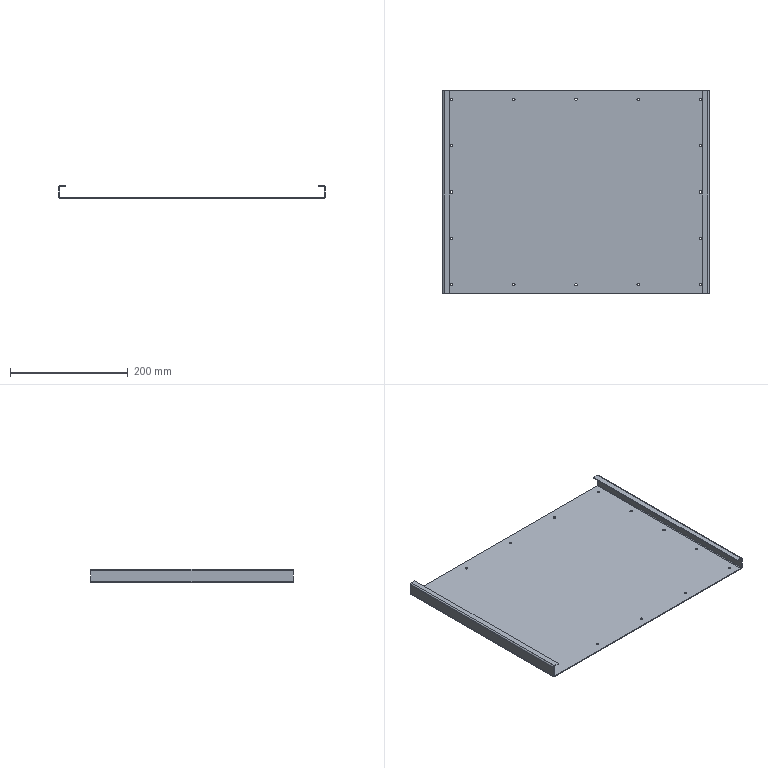Part | STEP file | Electrical box base plate 2 | 1 solid | 54 faces | box 453 x 345 x 23 mm | volume 265143 mm3 | plane 30 | cylinder 24 | commonest cylinder face diameters 4.2 x16 2 x4 5 x4
STEP:
#1=CARTESIAN_POINT('',(10.,345.,-1.));
#2=VERTEX_POINT('',#1);
#3=CARTESIAN_POINT('',(11.5,345.,-1.));
#4=VERTEX_POINT('',#3);
#5=CARTESIAN_POINT('',(10.,345.,-1.));
#6=DIRECTION('',(1.,0.,0.));
#7=VECTOR('',#6,1000.);
#8=LINE('',#5,#7);
#9=EDGE_CURVE('',#2,#4,#8,.T.);
#10=ORIENTED_EDGE('',*,*,#9,.F.);
#11=CARTESIAN_POINT('',(9.,345.,0.));
#12=VERTEX_POINT('',#11);
#13=CARTESIAN_POINT('',(9.,345.,-1.));
#14=DIRECTION('',(0.,1.,0.));
#15=DIRECTION('',(0.,0.,-1.));
#16=AXIS2_PLACEMENT_3D('',#13,#14,#15);
#17=CIRCLE('',#16,1.);
#18=EDGE_CURVE('',#12,#2,#17,.T.);
#19=ORIENTED_EDGE('',*,*,#18,.F.);
#20=CARTESIAN_POINT('',(9.,345.,1.5));
#21=VERTEX_POINT('',#20);
#22=CARTESIAN_POINT('',(9.,345.,1.5));
#23=DIRECTION('',(0.,0.,-1.));
#24=VECTOR('',#23,1000.);
#25=LINE('',#22,#24);
#26=EDGE_CURVE('',#21,#12,#25,.T.);
#27=ORIENTED_EDGE('',*,*,#26,.F.);
#28=CARTESIAN_POINT('',(9.,345.,-1.));
#29=DIRECTION('',(0.,1.,0.));
#30=DIRECTION('',(1.,0.,0.));
#31=AXIS2_PLACEMENT_3D('',#28,#29,#30);
#32=CIRCLE('',#31,2.5);
#33=EDGE_CURVE('',#21,#4,#32,.T.);
#34=ORIENTED_EDGE('',*,*,#33,.T.);
#35=EDGE_LOOP('',(#10,#19,#27,#34));
#36=FACE_OUTER_BOUND('',#35,.T.);
#37=CARTESIAN_POINT('',(10.,345.,-1.));
#38=DIRECTION('',(0.,1.,0.));
#39=DIRECTION('',(0.,0.,1.));
#40=AXIS2_PLACEMENT_3D('',#37,#38,#39);
#41=PLANE('',#40);
#42=ADVANCED_FACE('',(#36),#41,.T.);
#43=CARTESIAN_POINT('',(10.,345.,-19.));
#44=VERTEX_POINT('',#43);
#45=CARTESIAN_POINT('',(10.,345.,0.));
#46=DIRECTION('',(0.,0.,-1.));
#47=VECTOR('',#46,1000.);
#48=LINE('',#45,#47);
#49=EDGE_CURVE('',#2,#44,#48,.T.);
#50=ORIENTED_EDGE('',*,*,#49,.F.);
#51=ORIENTED_EDGE('',*,*,#9,.T.);
#52=CARTESIAN_POINT('',(11.5,345.,-19.));
#53=VERTEX_POINT('',#52);
#54=CARTESIAN_POINT('',(11.5,345.,0.));
#55=DIRECTION('',(0.,0.,-1.));
#56=VECTOR('',#55,1000.);
#57=LINE('',#54,#56);
#58=EDGE_CURVE('',#4,#53,#57,.T.);
#59=ORIENTED_EDGE('',*,*,#58,.T.);
#60=CARTESIAN_POINT('',(11.5,345.,-19.));
#61=DIRECTION('',(-1.,0.,0.));
#62=VECTOR('',#61,1000.);
#63=LINE('',#60,#62);
#64=EDGE_CURVE('',#53,#44,#63,.T.);
#65=ORIENTED_EDGE('',*,*,#64,.T.);
#66=EDGE_LOOP('',(#50,#51,#59,#65));
#67=FACE_OUTER_BOUND('',#66,.T.);
#68=CARTESIAN_POINT('',(9.,345.,1.5));
#69=DIRECTION('',(0.,1.,0.));
#70=DIRECTION('',(0.,0.,1.));
#71=AXIS2_PLACEMENT_3D('',#68,#69,#70);
#72=PLANE('',#71);
#73=ADVANCED_FACE('',(#67),#72,.T.);
#74=CARTESIAN_POINT('',(9.,0.,0.));
#75=VERTEX_POINT('',#74);
#76=CARTESIAN_POINT('',(9.,0.,1.5));
#77=VERTEX_POINT('',#76);
#78=CARTESIAN_POINT('',(9.,0.,0.));
#79=DIRECTION('',(0.,0.,1.));
#80=VECTOR('',#79,1000.);
#81=LINE('',#78,#80);
#82=EDGE_CURVE('',#75,#77,#81,.T.);
#83=ORIENTED_EDGE('',*,*,#82,.F.);
#84=CARTESIAN_POINT('',(10.,0.,-1.));
#85=VERTEX_POINT('',#84);
#86=CARTESIAN_POINT('',(9.,0.,-1.));
#87=DIRECTION('',(0.,1.,0.));
#88=DIRECTION('',(0.,0.,-1.));
#89=AXIS2_PLACEMENT_3D('',#86,#87,#88);
#90=CIRCLE('',#89,1.);
#91=EDGE_CURVE('',#75,#85,#90,.T.);
#92=ORIENTED_EDGE('',*,*,#91,.T.);
#93=CARTESIAN_POINT('',(11.5,0.,-1.));
#94=VERTEX_POINT('',#93);
#95=CARTESIAN_POINT('',(11.5,0.,-1.));
#96=DIRECTION('',(-1.,0.,0.));
#97=VECTOR('',#96,1000.);
#98=LINE('',#95,#97);
#99=EDGE_CURVE('',#94,#85,#98,.T.);
#100=ORIENTED_EDGE('',*,*,#99,.F.);
#101=CARTESIAN_POINT('',(9.,0.,-1.));
#102=DIRECTION('',(0.,1.,0.));
#103=DIRECTION('',(1.,0.,0.));
#104=AXIS2_PLACEMENT_3D('',#101,#102,#103);
#105=CIRCLE('',#104,2.5);
#106=EDGE_CURVE('',#77,#94,#105,.T.);
#107=ORIENTED_EDGE('',*,*,#106,.F.);
#108=EDGE_LOOP('',(#83,#92,#100,#107));
#109=FACE_OUTER_BOUND('',#108,.T.);
#110=CARTESIAN_POINT('',(9.,0.,0.));
#111=DIRECTION('',(0.,-1.,0.));
#112=DIRECTION('',(0.,0.,-1.));
#113=AXIS2_PLACEMENT_3D('',#110,#111,#112);
#114=PLANE('',#113);
#115=ADVANCED_FACE('',(#109),#114,.T.);
#116=CARTESIAN_POINT('',(0.,0.,0.));
#117=VERTEX_POINT('',#116);
#118=CARTESIAN_POINT('',(0.,0.,0.));
#119=DIRECTION('',(1.,0.,0.));
#120=VECTOR('',#119,1000.);
#121=LINE('',#118,#120);
#122=EDGE_CURVE('',#117,#75,#121,.T.);
#123=ORIENTED_EDGE('',*,*,#122,.T.);
#124=ORIENTED_EDGE('',*,*,#82,.T.);
#125=CARTESIAN_POINT('',(0.,0.,1.5));
#126=VERTEX_POINT('',#125);
#127=CARTESIAN_POINT('',(0.,0.,1.5));
#128=DIRECTION('',(1.,0.,0.));
#129=VECTOR('',#128,1000.);
#130=LINE('',#127,#129);
#131=EDGE_CURVE('',#126,#77,#130,.T.);
#132=ORIENTED_EDGE('',*,*,#131,.F.);
#133=CARTESIAN_POINT('',(0.,0.,1.5));
#134=DIRECTION('',(0.,0.,-1.));
#135=VECTOR('',#134,1000.);
#136=LINE('',#133,#135);
#137=EDGE_CURVE('',#126,#117,#136,.T.);
#138=ORIENTED_EDGE('',*,*,#137,.T.);
#139=EDGE_LOOP('',(#123,#124,#132,#138));
#140=FACE_OUTER_BOUND('',#139,.T.);
#141=CARTESIAN_POINT('',(11.5,0.,-1.));
#142=DIRECTION('',(0.,-1.,0.));
#143=DIRECTION('',(0.,0.,-1.));
#144=AXIS2_PLACEMENT_3D('',#141,#142,#143);
#145=PLANE('',#144);
#146=ADVANCED_FACE('',(#140),#145,.T.);
#147=CARTESIAN_POINT('',(9.,345.,-20.));
#148=VERTEX_POINT('',#147);
#149=CARTESIAN_POINT('',(9.,345.,-21.5));
#150=VERTEX_POINT('',#149);
#151=CARTESIAN_POINT('',(9.,345.,-20.));
#152=DIRECTION('',(0.,0.,-1.));
#153=VECTOR('',#152,1000.);
#154=LINE('',#151,#153);
#155=EDGE_CURVE('',#148,#150,#154,.T.);
#156=ORIENTED_EDGE('',*,*,#155,.F.);
#157=CARTESIAN_POINT('',(9.,345.,-19.));
#158=DIRECTION('',(0.,1.,0.));
#159=DIRECTION('',(0.,0.,-1.));
#160=AXIS2_PLACEMENT_3D('',#157,#158,#159);
#161=CIRCLE('',#160,1.);
#162=EDGE_CURVE('',#44,#148,#161,.T.);
#163=ORIENTED_EDGE('',*,*,#162,.F.);
#164=ORIENTED_EDGE('',*,*,#64,.F.);
#165=CARTESIAN_POINT('',(9.,345.,-19.));
#166=DIRECTION('',(0.,1.,0.));
#167=DIRECTION('',(1.,0.,0.));
#168=AXIS2_PLACEMENT_3D('',#165,#166,#167);
#169=CIRCLE('',#168,2.5);
#170=EDGE_CURVE('',#53,#150,#169,.T.);
#171=ORIENTED_EDGE('',*,*,#170,.T.);
#172=EDGE_LOOP('',(#156,#163,#164,#171));
#173=FACE_OUTER_BOUND('',#172,.T.);
#174=CARTESIAN_POINT('',(9.,345.,-20.));
#175=DIRECTION('',(0.,1.,0.));
#176=DIRECTION('',(0.,0.,1.));
#177=AXIS2_PLACEMENT_3D('',#174,#175,#176);
#178=PLANE('',#177);
#179=ADVANCED_FACE('',(#173),#178,.T.);
#180=CARTESIAN_POINT('',(-439.,345.,-20.));
#181=VERTEX_POINT('',#180);
#182=CARTESIAN_POINT('',(10.,345.,-20.));
#183=DIRECTION('',(-1.,0.,0.));
#184=VECTOR('',#183,1000.);
#185=LINE('',#182,#184);
#186=EDGE_CURVE('',#148,#181,#185,.T.);
#187=ORIENTED_EDGE('',*,*,#186,.F.);
#188=ORIENTED_EDGE('',*,*,#155,.T.);
#189=CARTESIAN_POINT('',(-439.,345.,-21.5));
#190=VERTEX_POINT('',#189);
#191=CARTESIAN_POINT('',(10.,345.,-21.5));
#192=DIRECTION('',(-1.,0.,0.));
#193=VECTOR('',#192,1000.);
#194=LINE('',#191,#193);
#195=EDGE_CURVE('',#150,#190,#194,.T.);
#196=ORIENTED_EDGE('',*,*,#195,.T.);
#197=CARTESIAN_POINT('',(-439.,345.,-21.5));
#198=DIRECTION('',(0.,0.,1.));
#199=VECTOR('',#198,1000.);
#200=LINE('',#197,#199);
#201=EDGE_CURVE('',#190,#181,#200,.T.);
#202=ORIENTED_EDGE('',*,*,#201,.T.);
#203=EDGE_LOOP('',(#187,#188,#196,#202));
#204=FACE_OUTER_BOUND('',#203,.T.);
#205=CARTESIAN_POINT('',(11.5,345.,-19.));
#206=DIRECTION('',(0.,1.,0.));
#207=DIRECTION('',(0.,0.,1.));
#208=AXIS2_PLACEMENT_3D('',#205,#206,#207);
#209=PLANE('',#208);
#210=ADVANCED_FACE('',(#204),#209,.T.);
#211=CARTESIAN_POINT('',(10.,0.,-19.));
#212=VERTEX_POINT('',#211);
#213=CARTESIAN_POINT('',(11.5,0.,-19.));
#214=VERTEX_POINT('',#213);
#215=CARTESIAN_POINT('',(10.,0.,-19.));
#216=DIRECTION('',(1.,0.,0.));
#217=VECTOR('',#216,1000.);
#218=LINE('',#215,#217);
#219=EDGE_CURVE('',#212,#214,#218,.T.);
#220=ORIENTED_EDGE('',*,*,#219,.F.);
#221=CARTESIAN_POINT('',(9.,0.,-20.));
#222=VERTEX_POINT('',#221);
#223=CARTESIAN_POINT('',(9.,0.,-19.));
#224=DIRECTION('',(0.,1.,0.));
#225=DIRECTION('',(0.,0.,-1.));
#226=AXIS2_PLACEMENT_3D('',#223,#224,#225);
#227=CIRCLE('',#226,1.);
#228=EDGE_CURVE('',#212,#222,#227,.T.);
#229=ORIENTED_EDGE('',*,*,#228,.T.);
#230=CARTESIAN_POINT('',(9.,0.,-21.5));
#231=VERTEX_POINT('',#230);
#232=CARTESIAN_POINT('',(9.,0.,-21.5));
#233=DIRECTION('',(0.,0.,1.));
#234=VECTOR('',#233,1000.);
#235=LINE('',#232,#234);
#236=EDGE_CURVE('',#231,#222,#235,.T.);
#237=ORIENTED_EDGE('',*,*,#236,.F.);
#238=CARTESIAN_POINT('',(9.,0.,-19.));
#239=DIRECTION('',(0.,1.,0.));
#240=DIRECTION('',(1.,0.,0.));
#241=AXIS2_PLACEMENT_3D('',#238,#239,#240);
#242=CIRCLE('',#241,2.5);
#243=EDGE_CURVE('',#214,#231,#242,.T.);
#244=ORIENTED_EDGE('',*,*,#243,.F.);
#245=EDGE_LOOP('',(#220,#229,#237,#244));
#246=FACE_OUTER_BOUND('',#245,.T.);
#247=CARTESIAN_POINT('',(10.,0.,-19.));
#248=DIRECTION('',(0.,-1.,0.));
#249=DIRECTION('',(0.,0.,-1.));
#250=AXIS2_PLACEMENT_3D('',#247,#248,#249);
#251=PLANE('',#250);
#252=ADVANCED_FACE('',(#246),#251,.T.);
#253=CARTESIAN_POINT('',(10.,0.,0.));
#254=DIRECTION('',(0.,0.,-1.));
#255=VECTOR('',#254,1000.);
#256=LINE('',#253,#255);
#257=EDGE_CURVE('',#85,#212,#256,.T.);
#258=ORIENTED_EDGE('',*,*,#257,.T.);
#259=ORIENTED_EDGE('',*,*,#219,.T.);
#260=CARTESIAN_POINT('',(11.5,0.,0.));
#261=DIRECTION('',(0.,0.,-1.));
#262=VECTOR('',#261,1000.);
#263=LINE('',#260,#262);
#264=EDGE_CURVE('',#94,#214,#263,.T.);
#265=ORIENTED_EDGE('',*,*,#264,.F.);
#266=ORIENTED_EDGE('',*,*,#99,.T.);
#267=EDGE_LOOP('',(#258,#259,#265,#266));
#268=FACE_OUTER_BOUND('',#267,.T.);
#269=CARTESIAN_POINT('',(9.,0.,-21.5));
#270=DIRECTION('',(0.,-1.,0.));
#271=DIRECTION('',(0.,0.,-1.));
#272=AXIS2_PLACEMENT_3D('',#269,#270,#271);
#273=PLANE('',#272);
#274=ADVANCED_FACE('',(#268),#273,.T.);
#275=CARTESIAN_POINT('',(-440.,345.,-19.));
#276=VERTEX_POINT('',#275);
#277=CARTESIAN_POINT('',(-441.5,345.,-19.));
#278=VERTEX_POINT('',#277);
#279=CARTESIAN_POINT('',(-440.,345.,-19.));
#280=DIRECTION('',(-1.,0.,0.));
#281=VECTOR('',#280,1000.);
#282=LINE('',#279,#281);
#283=EDGE_CURVE('',#276,#278,#282,.T.);
#284=ORIENTED_EDGE('',*,*,#283,.F.);
#285=CARTESIAN_POINT('',(-439.,345.,-19.));
#286=DIRECTION('',(0.,1.,0.));
#287=DIRECTION('',(0.,0.,-1.));
#288=AXIS2_PLACEMENT_3D('',#285,#286,#287);
#289=CIRCLE('',#288,1.);
#290=EDGE_CURVE('',#181,#276,#289,.T.);
#291=ORIENTED_EDGE('',*,*,#290,.F.);
#292=ORIENTED_EDGE('',*,*,#201,.F.);
#293=CARTESIAN_POINT('',(-439.,345.,-19.));
#294=DIRECTION('',(0.,1.,0.));
#295=DIRECTION('',(1.,0.,0.));
#296=AXIS2_PLACEMENT_3D('',#293,#294,#295);
#297=CIRCLE('',#296,2.5);
#298=EDGE_CURVE('',#190,#278,#297,.T.);
#299=ORIENTED_EDGE('',*,*,#298,.T.);
#300=EDGE_LOOP('',(#284,#291,#292,#299));
#301=FACE_OUTER_BOUND('',#300,.T.);
#302=CARTESIAN_POINT('',(-440.,345.,-19.));
#303=DIRECTION('',(0.,1.,0.));
#304=DIRECTION('',(0.,0.,1.));
#305=AXIS2_PLACEMENT_3D('',#302,#303,#304);
#306=PLANE('',#305);
#307=ADVANCED_FACE('',(#301),#306,.T.);
#308=CARTESIAN_POINT('',(-440.,345.,-1.));
#309=VERTEX_POINT('',#308);
#310=CARTESIAN_POINT('',(-440.,345.,-20.));
#311=DIRECTION('',(0.,0.,1.));
#312=VECTOR('',#311,1000.);
#313=LINE('',#310,#312);
#314=EDGE_CURVE('',#276,#309,#313,.T.);
#315=ORIENTED_EDGE('',*,*,#314,.F.);
#316=ORIENTED_EDGE('',*,*,#283,.T.);
#317=CARTESIAN_POINT('',(-441.5,345.,-1.));
#318=VERTEX_POINT('',#317);
#319=CARTESIAN_POINT('',(-441.5,345.,-20.));
#320=DIRECTION('',(0.,0.,1.));
#321=VECTOR('',#320,1000.);
#322=LINE('',#319,#321);
#323=EDGE_CURVE('',#278,#318,#322,.T.);
#324=ORIENTED_EDGE('',*,*,#323,.T.);
#325=CARTESIAN_POINT('',(-441.5,345.,-1.));
#326=DIRECTION('',(1.,0.,0.));
#327=VECTOR('',#326,1000.);
#328=LINE('',#325,#327);
#329=EDGE_CURVE('',#318,#309,#328,.T.);
#330=ORIENTED_EDGE('',*,*,#329,.T.);
#331=EDGE_LOOP('',(#315,#316,#324,#330));
#332=FACE_OUTER_BOUND('',#331,.T.);
#333=CARTESIAN_POINT('',(-439.,345.,-21.5));
#334=DIRECTION('',(0.,1.,0.));
#335=DIRECTION('',(0.,0.,1.));
#336=AXIS2_PLACEMENT_3D('',#333,#334,#335);
#337=PLANE('',#336);
#338=ADVANCED_FACE('',(#332),#337,.T.);
#339=CARTESIAN_POINT('',(-439.,0.,-20.));
#340=VERTEX_POINT('',#339);
#341=CARTESIAN_POINT('',(-439.,0.,-21.5));
#342=VERTEX_POINT('',#341);
#343=CARTESIAN_POINT('',(-439.,0.,-20.));
#344=DIRECTION('',(0.,0.,-1.));
#345=VECTOR('',#344,1000.);
#346=LINE('',#343,#345);
#347=EDGE_CURVE('',#340,#342,#346,.T.);
#348=ORIENTED_EDGE('',*,*,#347,.F.);
#349=CARTESIAN_POINT('',(-440.,0.,-19.));
#350=VERTEX_POINT('',#349);
#351=CARTESIAN_POINT('',(-439.,0.,-19.));
#352=DIRECTION('',(0.,1.,0.));
#353=DIRECTION('',(0.,0.,-1.));
#354=AXIS2_PLACEMENT_3D('',#351,#352,#353);
#355=CIRCLE('',#354,1.);
#356=EDGE_CURVE('',#340,#350,#355,.T.);
#357=ORIENTED_EDGE('',*,*,#356,.T.);
#358=CARTESIAN_POINT('',(-441.5,0.,-19.));
#359=VERTEX_POINT('',#358);
#360=CARTESIAN_POINT('',(-441.5,0.,-19.));
#361=DIRECTION('',(1.,0.,0.));
#362=VECTOR('',#361,1000.);
#363=LINE('',#360,#362);
#364=EDGE_CURVE('',#359,#350,#363,.T.);
#365=ORIENTED_EDGE('',*,*,#364,.F.);
#366=CARTESIAN_POINT('',(-439.,0.,-19.));
#367=DIRECTION('',(0.,1.,0.));
#368=DIRECTION('',(1.,0.,0.));
#369=AXIS2_PLACEMENT_3D('',#366,#367,#368);
#370=CIRCLE('',#369,2.5);
#371=EDGE_CURVE('',#342,#359,#370,.T.);
#372=ORIENTED_EDGE('',*,*,#371,.F.);
#373=EDGE_LOOP('',(#348,#357,#365,#372));
#374=FACE_OUTER_BOUND('',#373,.T.);
#375=CARTESIAN_POINT('',(-439.,0.,-20.));
#376=DIRECTION('',(0.,-1.,0.));
#377=DIRECTION('',(0.,0.,-1.));
#378=AXIS2_PLACEMENT_3D('',#375,#376,#377);
#379=PLANE('',#378);
#380=ADVANCED_FACE('',(#374),#379,.T.);
#381=CARTESIAN_POINT('',(10.,0.,-20.));
#382=DIRECTION('',(-1.,0.,0.));
#383=VECTOR('',#382,1000.);
#384=LINE('',#381,#383);
#385=EDGE_CURVE('',#222,#340,#384,.T.);
#386=ORIENTED_EDGE('',*,*,#385,.T.);
#387=ORIENTED_EDGE('',*,*,#347,.T.);
#388=CARTESIAN_POINT('',(10.,0.,-21.5));
#389=DIRECTION('',(-1.,0.,0.));
#390=VECTOR('',#389,1000.);
#391=LINE('',#388,#390);
#392=EDGE_CURVE('',#231,#342,#391,.T.);
#393=ORIENTED_EDGE('',*,*,#392,.F.);
#394=ORIENTED_EDGE('',*,*,#236,.T.);
#395=EDGE_LOOP('',(#386,#387,#393,#394));
#396=FACE_OUTER_BOUND('',#395,.T.);
#397=CARTESIAN_POINT('',(-441.5,0.,-19.));
#398=DIRECTION('',(0.,-1.,0.));
#399=DIRECTION('',(0.,0.,-1.));
#400=AXIS2_PLACEMENT_3D('',#397,#398,#399);
#401=PLANE('',#400);
#402=ADVANCED_FACE('',(#396),#401,.T.);
#403=CARTESIAN_POINT('',(-439.,345.,0.));
#404=VERTEX_POINT('',#403);
#405=CARTESIAN_POINT('',(-439.,345.,1.5));
#406=VERTEX_POINT('',#405);
#407=CARTESIAN_POINT('',(-439.,345.,0.));
#408=DIRECTION('',(0.,0.,1.));
#409=VECTOR('',#408,1000.);
#410=LINE('',#407,#409);
#411=EDGE_CURVE('',#404,#406,#410,.T.);
#412=ORIENTED_EDGE('',*,*,#411,.F.);
#413=CARTESIAN_POINT('',(-439.,345.,-1.));
#414=DIRECTION('',(0.,1.,0.));
#415=DIRECTION('',(0.,0.,-1.));
#416=AXIS2_PLACEMENT_3D('',#413,#414,#415);
#417=CIRCLE('',#416,1.);
#418=EDGE_CURVE('',#309,#404,#417,.T.);
#419=ORIENTED_EDGE('',*,*,#418,.F.);
#420=ORIENTED_EDGE('',*,*,#329,.F.);
#421=CARTESIAN_POINT('',(-439.,345.,-1.));
#422=DIRECTION('',(0.,1.,0.));
#423=DIRECTION('',(1.,0.,0.));
#424=AXIS2_PLACEMENT_3D('',#421,#422,#423);
#425=CIRCLE('',#424,2.5);
#426=EDGE_CURVE('',#318,#406,#425,.T.);
#427=ORIENTED_EDGE('',*,*,#426,.T.);
#428=EDGE_LOOP('',(#412,#419,#420,#427));
#429=FACE_OUTER_BOUND('',#428,.T.);
#430=CARTESIAN_POINT('',(-439.,345.,0.));
#431=DIRECTION('',(0.,1.,0.));
#432=DIRECTION('',(0.,0.,1.));
#433=AXIS2_PLACEMENT_3D('',#430,#431,#432);
#434=PLANE('',#433);
#435=ADVANCED_FACE('',(#429),#434,.T.);
#436=CARTESIAN_POINT('',(-430.,345.,0.));
#437=VERTEX_POINT('',#436);
#438=CARTESIAN_POINT('',(-440.,345.,0.));
#439=DIRECTION('',(1.,0.,0.));
#440=VECTOR('',#439,1000.);
#441=LINE('',#438,#440);
#442=EDGE_CURVE('',#404,#437,#441,.T.);
#443=ORIENTED_EDGE('',*,*,#442,.F.);
#444=ORIENTED_EDGE('',*,*,#411,.T.);
#445=CARTESIAN_POINT('',(-430.,345.,1.5));
#446=VERTEX_POINT('',#445);
#447=CARTESIAN_POINT('',(-440.,345.,1.5));
#448=DIRECTION('',(1.,0.,0.));
#449=VECTOR('',#448,1000.);
#450=LINE('',#447,#449);
#451=EDGE_CURVE('',#406,#446,#450,.T.);
#452=ORIENTED_EDGE('',*,*,#451,.T.);
#453=CARTESIAN_POINT('',(-430.,345.,0.));
#454=DIRECTION('',(0.,0.,1.));
#455=VECTOR('',#454,1000.);
#456=LINE('',#453,#455);
#457=EDGE_CURVE('',#437,#446,#456,.T.);
#458=ORIENTED_EDGE('',*,*,#457,.F.);
#459=EDGE_LOOP('',(#443,#444,#452,#458));
#460=FACE_OUTER_BOUND('',#459,.T.);
#461=CARTESIAN_POINT('',(-441.5,345.,-1.));
#462=DIRECTION('',(0.,1.,0.));
#463=DIRECTION('',(0.,0.,1.));
#464=AXIS2_PLACEMENT_3D('',#461,#462,#463);
#465=PLANE('',#464);
#466=ADVANCED_FACE('',(#460),#465,.T.);
#467=CARTESIAN_POINT('',(-440.,0.,-1.));
#468=VERTEX_POINT('',#467);
#469=CARTESIAN_POINT('',(-441.5,0.,-1.));
#470=VERTEX_POINT('',#469);
#471=CARTESIAN_POINT('',(-440.,0.,-1.));
#472=DIRECTION('',(-1.,0.,0.));
#473=VECTOR('',#472,1000.);
#474=LINE('',#471,#473);
#475=EDGE_CURVE('',#468,#470,#474,.T.);
#476=ORIENTED_EDGE('',*,*,#475,.F.);
#477=CARTESIAN_POINT('',(-439.,0.,0.));
#478=VERTEX_POINT('',#477);
#479=CARTESIAN_POINT('',(-439.,0.,-1.));
#480=DIRECTION('',(0.,1.,0.));
#481=DIRECTION('',(0.,0.,-1.));
#482=AXIS2_PLACEMENT_3D('',#479,#480,#481);
#483=CIRCLE('',#482,1.);
#484=EDGE_CURVE('',#468,#478,#483,.T.);
#485=ORIENTED_EDGE('',*,*,#484,.T.);
#486=CARTESIAN_POINT('',(-439.,0.,1.5));
#487=VERTEX_POINT('',#486);
#488=CARTESIAN_POINT('',(-439.,0.,1.5));
#489=DIRECTION('',(0.,0.,-1.));
#490=VECTOR('',#489,1000.);
#491=LINE('',#488,#490);
#492=EDGE_CURVE('',#487,#478,#491,.T.);
#493=ORIENTED_EDGE('',*,*,#492,.F.);
#494=CARTESIAN_POINT('',(-439.,0.,-1.));
#495=DIRECTION('',(0.,1.,0.));
#496=DIRECTION('',(1.,0.,0.));
#497=AXIS2_PLACEMENT_3D('',#494,#495,#496);
#498=CIRCLE('',#497,2.5);
#499=EDGE_CURVE('',#470,#487,#498,.T.);
#500=ORIENTED_EDGE('',*,*,#499,.F.);
#501=EDGE_LOOP('',(#476,#485,#493,#500));
#502=FACE_OUTER_BOUND('',#501,.T.);
#503=CARTESIAN_POINT('',(-440.,0.,-1.));
#504=DIRECTION('',(0.,-1.,0.));
#505=DIRECTION('',(0.,0.,-1.));
#506=AXIS2_PLACEMENT_3D('',#503,#504,#505);
#507=PLANE('',#506);
#508=ADVANCED_FACE('',(#502),#507,.T.);
#509=CARTESIAN_POINT('',(-440.,0.,-20.));
#510=DIRECTION('',(0.,0.,1.));
#511=VECTOR('',#510,1000.);
#512=LINE('',#509,#511);
#513=EDGE_CURVE('',#350,#468,#512,.T.);
#514=ORIENTED_EDGE('',*,*,#513,.T.);
#515=ORIENTED_EDGE('',*,*,#475,.T.);
#516=CARTESIAN_POINT('',(-441.5,0.,-20.));
#517=DIRECTION('',(0.,0.,1.));
#518=VECTOR('',#517,1000.);
#519=LINE('',#516,#518);
#520=EDGE_CURVE('',#359,#470,#519,.T.);
#521=ORIENTED_EDGE('',*,*,#520,.F.);
#522=ORIENTED_EDGE('',*,*,#364,.T.);
#523=EDGE_LOOP('',(#514,#515,#521,#522));
#524=FACE_OUTER_BOUND('',#523,.T.);
#525=CARTESIAN_POINT('',(-439.,0.,1.5));
#526=DIRECTION('',(0.,-1.,0.));
#527=DIRECTION('',(0.,0.,-1.));
#528=AXIS2_PLACEMENT_3D('',#525,#526,#527);
#529=PLANE('',#528);
#530=ADVANCED_FACE('',(#524),#529,.T.);
#531=CARTESIAN_POINT('',(-430.,0.,1.5));
#532=VERTEX_POINT('',#531);
#533=CARTESIAN_POINT('',(-440.,0.,1.5));
#534=DIRECTION('',(1.,0.,0.));
#535=VECTOR('',#534,1000.);
#536=LINE('',#533,#535);
#537=EDGE_CURVE('',#487,#532,#536,.T.);
#538=ORIENTED_EDGE('',*,*,#537,.T.);
#539=CARTESIAN_POINT('',(-430.,345.,1.5));
#540=DIRECTION('',(0.,-1.,0.));
#541=VECTOR('',#540,1000.);
#542=LINE('',#539,#541);
#543=EDGE_CURVE('',#446,#532,#542,.T.);
#544=ORIENTED_EDGE('',*,*,#543,.F.);
#545=ORIENTED_EDGE('',*,*,#451,.F.);
#546=CARTESIAN_POINT('',(-439.,345.,1.5));
#547=DIRECTION('',(0.,-1.,0.));
#548=VECTOR('',#547,1000.);
#549=LINE('',#546,#548);
#550=EDGE_CURVE('',#406,#487,#549,.T.);
#551=ORIENTED_EDGE('',*,*,#550,.T.);
#552=EDGE_LOOP('',(#538,#544,#545,#551));
#553=FACE_OUTER_BOUND('',#552,.T.);
#554=CARTESIAN_POINT('',(-440.,345.,1.5));
#555=DIRECTION('',(0.,0.,-1.));
#556=DIRECTION('',(-1.,0.,0.));
#557=AXIS2_PLACEMENT_3D('',#554,#555,#556);
#558=PLANE('',#557);
#559=ADVANCED_FACE('',(#553),#558,.F.);
#560=CARTESIAN_POINT('',(-430.,0.,0.));
#561=VERTEX_POINT('',#560);
#562=CARTESIAN_POINT('',(-430.,0.,0.));
#563=DIRECTION('',(0.,0.,1.));
#564=VECTOR('',#563,1000.);
#565=LINE('',#562,#564);
#566=EDGE_CURVE('',#561,#532,#565,.T.);
#567=ORIENTED_EDGE('',*,*,#566,.F.);
#568=CARTESIAN_POINT('',(-430.,345.,0.));
#569=DIRECTION('',(0.,-1.,0.));
#570=VECTOR('',#569,1000.);
#571=LINE('',#568,#570);
#572=EDGE_CURVE('',#437,#561,#571,.T.);
#573=ORIENTED_EDGE('',*,*,#572,.F.);
#574=ORIENTED_EDGE('',*,*,#457,.T.);
#575=ORIENTED_EDGE('',*,*,#543,.T.);
#576=EDGE_LOOP('',(#567,#573,#574,#575));
#577=FACE_OUTER_BOUND('',#576,.T.);
#578=CARTESIAN_POINT('',(-430.,345.,0.));
#579=DIRECTION('',(1.,0.,0.));
#580=DIRECTION('',(0.,0.,-1.));
#581=AXIS2_PLACEMENT_3D('',#578,#579,#580);
#582=PLANE('',#581);
#583=ADVANCED_FACE('',(#577),#582,.T.);
#584=CARTESIAN_POINT('',(-440.,0.,0.));
#585=DIRECTION('',(1.,0.,0.));
#586=VECTOR('',#585,1000.);
#587=LINE('',#584,#586);
#588=EDGE_CURVE('',#478,#561,#587,.T.);
#589=ORIENTED_EDGE('',*,*,#588,.F.);
#590=CARTESIAN_POINT('',(-439.,345.,0.));
#591=DIRECTION('',(0.,-1.,0.));
#592=VECTOR('',#591,1000.);
#593=LINE('',#590,#592);
#594=EDGE_CURVE('',#404,#478,#593,.T.);
#595=ORIENTED_EDGE('',*,*,#594,.F.);
#596=ORIENTED_EDGE('',*,*,#442,.T.);
#597=ORIENTED_EDGE('',*,*,#572,.T.);
#598=EDGE_LOOP('',(#589,#595,#596,#597));
#599=FACE_OUTER_BOUND('',#598,.T.);
#600=CARTESIAN_POINT('',(-440.,345.,0.));
#601=DIRECTION('',(0.,0.,-1.));
#602=DIRECTION('',(-1.,0.,0.));
#603=AXIS2_PLACEMENT_3D('',#600,#601,#602);
#604=PLANE('',#603);
#605=ADVANCED_FACE('',(#599),#604,.T.);
#606=ORIENTED_EDGE('',*,*,#484,.F.);
#607=CARTESIAN_POINT('',(-440.,345.,-1.));
#608=DIRECTION('',(0.,-1.,0.));
#609=VECTOR('',#608,1000.);
#610=LINE('',#607,#609);
#611=EDGE_CURVE('',#309,#468,#610,.T.);
#612=ORIENTED_EDGE('',*,*,#611,.F.);
#613=ORIENTED_EDGE('',*,*,#418,.T.);
#614=ORIENTED_EDGE('',*,*,#594,.T.);
#615=EDGE_LOOP('',(#606,#612,#613,#614));
#616=FACE_OUTER_BOUND('',#615,.T.);
#617=CARTESIAN_POINT('',(-439.,345.,-1.));
#618=DIRECTION('',(0.,-1.,0.));
#619=DIRECTION('',(0.,0.,-1.));
#620=AXIS2_PLACEMENT_3D('',#617,#618,#619);
#621=CYLINDRICAL_SURFACE('',#620,1.);
#622=ADVANCED_FACE('',(#616),#621,.F.);
#623=ORIENTED_EDGE('',*,*,#513,.F.);
#624=CARTESIAN_POINT('',(-440.,345.,-19.));
#625=DIRECTION('',(0.,-1.,0.));
#626=VECTOR('',#625,1000.);
#627=LINE('',#624,#626);
#628=EDGE_CURVE('',#276,#350,#627,.T.);
#629=ORIENTED_EDGE('',*,*,#628,.F.);
#630=ORIENTED_EDGE('',*,*,#314,.T.);
#631=ORIENTED_EDGE('',*,*,#611,.T.);
#632=EDGE_LOOP('',(#623,#629,#630,#631));
#633=FACE_OUTER_BOUND('',#632,.T.);
#634=CARTESIAN_POINT('',(-440.,345.,-20.));
#635=DIRECTION('',(1.,0.,0.));
#636=DIRECTION('',(0.,0.,-1.));
#637=AXIS2_PLACEMENT_3D('',#634,#635,#636);
#638=PLANE('',#637);
#639=ADVANCED_FACE('',(#633),#638,.T.);
#640=ORIENTED_EDGE('',*,*,#356,.F.);
#641=CARTESIAN_POINT('',(-439.,345.,-20.));
#642=DIRECTION('',(0.,-1.,0.));
#643=VECTOR('',#642,1000.);
#644=LINE('',#641,#643);
#645=EDGE_CURVE('',#181,#340,#644,.T.);
#646=ORIENTED_EDGE('',*,*,#645,.F.);
#647=ORIENTED_EDGE('',*,*,#290,.T.);
#648=ORIENTED_EDGE('',*,*,#628,.T.);
#649=EDGE_LOOP('',(#640,#646,#647,#648));
#650=FACE_OUTER_BOUND('',#649,.T.);
#651=CARTESIAN_POINT('',(-439.,345.,-19.));
#652=DIRECTION('',(0.,-1.,0.));
#653=DIRECTION('',(0.,0.,-1.));
#654=AXIS2_PLACEMENT_3D('',#651,#652,#653);
#655=CYLINDRICAL_SURFACE('',#654,1.);
#656=ADVANCED_FACE('',(#650),#655,.F.);
#657=CARTESIAN_POINT('',(-424.4,15.,-20.));
#658=VERTEX_POINT('',#657);
#659=CARTESIAN_POINT('',(-426.5,15.,-20.));
#660=DIRECTION('',(0.,0.,1.));
#661=DIRECTION('',(1.,0.,0.));
#662=AXIS2_PLACEMENT_3D('',#659,#660,#661);
#663=CIRCLE('',#662,2.1);
#664=EDGE_CURVE('',#658,#658,#663,.T.);
#665=ORIENTED_EDGE('',*,*,#664,.F.);
#666=EDGE_LOOP('',(#665));
#667=FACE_BOUND('',#666,.T.);
#668=CARTESIAN_POINT('',(-318.65,15.,-20.));
#669=VERTEX_POINT('',#668);
#670=CARTESIAN_POINT('',(-320.75,15.,-20.));
#671=DIRECTION('',(0.,0.,1.));
#672=DIRECTION('',(1.,0.,0.));
#673=AXIS2_PLACEMENT_3D('',#670,#671,#672);
#674=CIRCLE('',#673,2.1);
#675=EDGE_CURVE('',#669,#669,#674,.T.);
#676=ORIENTED_EDGE('',*,*,#675,.F.);
#677=EDGE_LOOP('',(#676));
#678=FACE_BOUND('',#677,.T.);
#679=CARTESIAN_POINT('',(-212.9,15.,-20.));
#680=VERTEX_POINT('',#679);
#681=CARTESIAN_POINT('',(-215.,15.,-20.));
#682=DIRECTION('',(0.,0.,1.));
#683=DIRECTION('',(1.,0.,0.));
#684=AXIS2_PLACEMENT_3D('',#681,#682,#683);
#685=CIRCLE('',#684,2.1);
#686=EDGE_CURVE('',#680,#680,#685,.T.);
#687=ORIENTED_EDGE('',*,*,#686,.F.);
#688=EDGE_LOOP('',(#687));
#689=FACE_BOUND('',#688,.T.);
#690=CARTESIAN_POINT('',(-107.15,15.,-20.));
#691=VERTEX_POINT('',#690);
#692=CARTESIAN_POINT('',(-109.25,15.,-20.));
#693=DIRECTION('',(0.,0.,1.));
#694=DIRECTION('',(1.,0.,0.));
#695=AXIS2_PLACEMENT_3D('',#692,#693,#694);
#696=CIRCLE('',#695,2.1);
#697=EDGE_CURVE('',#691,#691,#696,.T.);
#698=ORIENTED_EDGE('',*,*,#697,.F.);
#699=EDGE_LOOP('',(#698));
#700=FACE_BOUND('',#699,.T.);
#701=CARTESIAN_POINT('',(-1.4,15.,-20.));
#702=VERTEX_POINT('',#701);
#703=CARTESIAN_POINT('',(-3.5,15.,-20.));
#704=DIRECTION('',(0.,0.,1.));
#705=DIRECTION('',(1.,0.,0.));
#706=AXIS2_PLACEMENT_3D('',#703,#704,#705);
#707=CIRCLE('',#706,2.1);
#708=EDGE_CURVE('',#702,#702,#707,.T.);
#709=ORIENTED_EDGE('',*,*,#708,.F.);
#710=EDGE_LOOP('',(#709));
#711=FACE_BOUND('',#710,.T.);
#712=CARTESIAN_POINT('',(-1.4,330.,-20.));
#713=VERTEX_POINT('',#712);
#714=CARTESIAN_POINT('',(-3.5,330.,-20.));
#715=DIRECTION('',(0.,0.,1.));
#716=DIRECTION('',(1.,0.,0.));
#717=AXIS2_PLACEMENT_3D('',#714,#715,#716);
#718=CIRCLE('',#717,2.1);
#719=EDGE_CURVE('',#713,#713,#718,.T.);
#720=ORIENTED_EDGE('',*,*,#719,.F.);
#721=EDGE_LOOP('',(#720));
#722=FACE_BOUND('',#721,.T.);
#723=CARTESIAN_POINT('',(-107.15,330.,-20.));
#724=VERTEX_POINT('',#723);
#725=CARTESIAN_POINT('',(-109.25,330.,-20.));
#726=DIRECTION('',(0.,0.,1.));
#727=DIRECTION('',(1.,0.,0.));
#728=AXIS2_PLACEMENT_3D('',#725,#726,#727);
#729=CIRCLE('',#728,2.1);
#730=EDGE_CURVE('',#724,#724,#729,.T.);
#731=ORIENTED_EDGE('',*,*,#730,.F.);
#732=EDGE_LOOP('',(#731));
#733=FACE_BOUND('',#732,.T.);
#734=CARTESIAN_POINT('',(-212.9,330.,-20.));
#735=VERTEX_POINT('',#734);
#736=CARTESIAN_POINT('',(-215.,330.,-20.));
#737=DIRECTION('',(0.,0.,1.));
#738=DIRECTION('',(1.,0.,0.));
#739=AXIS2_PLACEMENT_3D('',#736,#737,#738);
#740=CIRCLE('',#739,2.1);
#741=EDGE_CURVE('',#735,#735,#740,.T.);
#742=ORIENTED_EDGE('',*,*,#741,.F.);
#743=EDGE_LOOP('',(#742));
#744=FACE_BOUND('',#743,.T.);
#745=CARTESIAN_POINT('',(-318.65,330.,-20.));
#746=VERTEX_POINT('',#745);
#747=CARTESIAN_POINT('',(-320.75,330.,-20.));
#748=DIRECTION('',(0.,0.,1.));
#749=DIRECTION('',(1.,0.,0.));
#750=AXIS2_PLACEMENT_3D('',#747,#748,#749);
#751=CIRCLE('',#750,2.1);
#752=EDGE_CURVE('',#746,#746,#751,.T.);
#753=ORIENTED_EDGE('',*,*,#752,.F.);
#754=EDGE_LOOP('',(#753));
#755=FACE_BOUND('',#754,.T.);
#756=CARTESIAN_POINT('',(-424.4,93.75,-20.));
#757=VERTEX_POINT('',#756);
#758=CARTESIAN_POINT('',(-426.5,93.75,-20.));
#759=DIRECTION('',(0.,0.,1.));
#760=DIRECTION('',(1.,0.,0.));
#761=AXIS2_PLACEMENT_3D('',#758,#759,#760);
#762=CIRCLE('',#761,2.1);
#763=EDGE_CURVE('',#757,#757,#762,.T.);
#764=ORIENTED_EDGE('',*,*,#763,.F.);
#765=EDGE_LOOP('',(#764));
#766=FACE_BOUND('',#765,.T.);
#767=CARTESIAN_POINT('',(-424.4,172.5,-20.));
#768=VERTEX_POINT('',#767);
#769=CARTESIAN_POINT('',(-426.5,172.5,-20.));
#770=DIRECTION('',(0.,0.,1.));
#771=DIRECTION('',(1.,0.,0.));
#772=AXIS2_PLACEMENT_3D('',#769,#770,#771);
#773=CIRCLE('',#772,2.1);
#774=EDGE_CURVE('',#768,#768,#773,.T.);
#775=ORIENTED_EDGE('',*,*,#774,.F.);
#776=EDGE_LOOP('',(#775));
#777=FACE_BOUND('',#776,.T.);
#778=CARTESIAN_POINT('',(-424.4,251.25,-20.));
#779=VERTEX_POINT('',#778);
#780=CARTESIAN_POINT('',(-426.5,251.25,-20.));
#781=DIRECTION('',(0.,0.,1.));
#782=DIRECTION('',(1.,0.,0.));
#783=AXIS2_PLACEMENT_3D('',#780,#781,#782);
#784=CIRCLE('',#783,2.1);
#785=EDGE_CURVE('',#779,#779,#784,.T.);
#786=ORIENTED_EDGE('',*,*,#785,.F.);
#787=EDGE_LOOP('',(#786));
#788=FACE_BOUND('',#787,.T.);
#789=CARTESIAN_POINT('',(-424.4,330.,-20.));
#790=VERTEX_POINT('',#789);
#791=CARTESIAN_POINT('',(-426.5,330.,-20.));
#792=DIRECTION('',(0.,0.,1.));
#793=DIRECTION('',(1.,0.,0.));
#794=AXIS2_PLACEMENT_3D('',#791,#792,#793);
#795=CIRCLE('',#794,2.1);
#796=EDGE_CURVE('',#790,#790,#795,.T.);
#797=ORIENTED_EDGE('',*,*,#796,.F.);
#798=EDGE_LOOP('',(#797));
#799=FACE_BOUND('',#798,.T.);
#800=CARTESIAN_POINT('',(-1.4,251.25,-20.));
#801=VERTEX_POINT('',#800);
#802=CARTESIAN_POINT('',(-3.5,251.25,-20.));
#803=DIRECTION('',(0.,0.,1.));
#804=DIRECTION('',(1.,0.,0.));
#805=AXIS2_PLACEMENT_3D('',#802,#803,#804);
#806=CIRCLE('',#805,2.1);
#807=EDGE_CURVE('',#801,#801,#806,.T.);
#808=ORIENTED_EDGE('',*,*,#807,.F.);
#809=EDGE_LOOP('',(#808));
#810=FACE_BOUND('',#809,.T.);
#811=CARTESIAN_POINT('',(-1.4,172.5,-20.));
#812=VERTEX_POINT('',#811);
#813=CARTESIAN_POINT('',(-3.5,172.5,-20.));
#814=DIRECTION('',(0.,0.,1.));
#815=DIRECTION('',(1.,0.,0.));
#816=AXIS2_PLACEMENT_3D('',#813,#814,#815);
#817=CIRCLE('',#816,2.1);
#818=EDGE_CURVE('',#812,#812,#817,.T.);
#819=ORIENTED_EDGE('',*,*,#818,.F.);
#820=EDGE_LOOP('',(#819));
#821=FACE_BOUND('',#820,.T.);
#822=CARTESIAN_POINT('',(-1.4,93.75,-20.));
#823=VERTEX_POINT('',#822);
#824=CARTESIAN_POINT('',(-3.5,93.75,-20.));
#825=DIRECTION('',(0.,0.,1.));
#826=DIRECTION('',(1.,0.,0.));
#827=AXIS2_PLACEMENT_3D('',#824,#825,#826);
#828=CIRCLE('',#827,2.1);
#829=EDGE_CURVE('',#823,#823,#828,.T.);
#830=ORIENTED_EDGE('',*,*,#829,.F.);
#831=EDGE_LOOP('',(#830));
#832=FACE_BOUND('',#831,.T.);
#833=ORIENTED_EDGE('',*,*,#385,.F.);
#834=CARTESIAN_POINT('',(9.,345.,-20.));
#835=DIRECTION('',(0.,-1.,0.));
#836=VECTOR('',#835,1000.);
#837=LINE('',#834,#836);
#838=EDGE_CURVE('',#148,#222,#837,.T.);
#839=ORIENTED_EDGE('',*,*,#838,.F.);
#840=ORIENTED_EDGE('',*,*,#186,.T.);
#841=ORIENTED_EDGE('',*,*,#645,.T.);
#842=EDGE_LOOP('',(#833,#839,#840,#841));
#843=FACE_OUTER_BOUND('',#842,.T.);
#844=CARTESIAN_POINT('',(10.,345.,-20.));
#845=DIRECTION('',(0.,0.,1.));
#846=DIRECTION('',(1.,0.,0.));
#847=AXIS2_PLACEMENT_3D('',#844,#845,#846);
#848=PLANE('',#847);
#849=ADVANCED_FACE('',(#667,#678,#689,#700,#711,#722,#733,#744,#755,#766,#777,#788,#799,#810,#821,#832,#843),#848,.T.);
#850=ORIENTED_EDGE('',*,*,#228,.F.);
#851=CARTESIAN_POINT('',(10.,345.,-19.));
#852=DIRECTION('',(0.,-1.,0.));
#853=VECTOR('',#852,1000.);
#854=LINE('',#851,#853);
#855=EDGE_CURVE('',#44,#212,#854,.T.);
#856=ORIENTED_EDGE('',*,*,#855,.F.);
#857=ORIENTED_EDGE('',*,*,#162,.T.);
#858=ORIENTED_EDGE('',*,*,#838,.T.);
#859=EDGE_LOOP('',(#850,#856,#857,#858));
#860=FACE_OUTER_BOUND('',#859,.T.);
#861=CARTESIAN_POINT('',(9.,345.,-19.));
#862=DIRECTION('',(0.,-1.,0.));
#863=DIRECTION('',(0.,0.,-1.));
#864=AXIS2_PLACEMENT_3D('',#861,#862,#863);
#865=CYLINDRICAL_SURFACE('',#864,1.);
#866=ADVANCED_FACE('',(#860),#865,.F.);
#867=ORIENTED_EDGE('',*,*,#257,.F.);
#868=CARTESIAN_POINT('',(10.,345.,-1.));
#869=DIRECTION('',(0.,-1.,0.));
#870=VECTOR('',#869,1000.);
#871=LINE('',#868,#870);
#872=EDGE_CURVE('',#2,#85,#871,.T.);
#873=ORIENTED_EDGE('',*,*,#872,.F.);
#874=ORIENTED_EDGE('',*,*,#49,.T.);
#875=ORIENTED_EDGE('',*,*,#855,.T.);
#876=EDGE_LOOP('',(#867,#873,#874,#875));
#877=FACE_OUTER_BOUND('',#876,.T.);
#878=CARTESIAN_POINT('',(10.,345.,0.));
#879=DIRECTION('',(-1.,0.,0.));
#880=DIRECTION('',(0.,0.,1.));
#881=AXIS2_PLACEMENT_3D('',#878,#879,#880);
#882=PLANE('',#881);
#883=ADVANCED_FACE('',(#877),#882,.T.);
#884=ORIENTED_EDGE('',*,*,#91,.F.);
#885=CARTESIAN_POINT('',(9.,345.,0.));
#886=DIRECTION('',(0.,-1.,0.));
#887=VECTOR('',#886,1000.);
#888=LINE('',#885,#887);
#889=EDGE_CURVE('',#12,#75,#888,.T.);
#890=ORIENTED_EDGE('',*,*,#889,.F.);
#891=ORIENTED_EDGE('',*,*,#18,.T.);
#892=ORIENTED_EDGE('',*,*,#872,.T.);
#893=EDGE_LOOP('',(#884,#890,#891,#892));
#894=FACE_OUTER_BOUND('',#893,.T.);
#895=CARTESIAN_POINT('',(9.,345.,-1.));
#896=DIRECTION('',(0.,-1.,0.));
#897=DIRECTION('',(0.,0.,-1.));
#898=AXIS2_PLACEMENT_3D('',#895,#896,#897);
#899=CYLINDRICAL_SURFACE('',#898,1.);
#900=ADVANCED_FACE('',(#894),#899,.F.);
#901=ORIENTED_EDGE('',*,*,#122,.F.);
#902=CARTESIAN_POINT('',(0.,345.,0.));
#903=VERTEX_POINT('',#902);
#904=CARTESIAN_POINT('',(0.,345.,0.));
#905=DIRECTION('',(0.,-1.,0.));
#906=VECTOR('',#905,1000.);
#907=LINE('',#904,#906);
#908=EDGE_CURVE('',#903,#117,#907,.T.);
#909=ORIENTED_EDGE('',*,*,#908,.F.);
#910=CARTESIAN_POINT('',(0.,345.,0.));
#911=DIRECTION('',(1.,0.,0.));
#912=VECTOR('',#911,1000.);
#913=LINE('',#910,#912);
#914=EDGE_CURVE('',#903,#12,#913,.T.);
#915=ORIENTED_EDGE('',*,*,#914,.T.);
#916=ORIENTED_EDGE('',*,*,#889,.T.);
#917=EDGE_LOOP('',(#901,#909,#915,#916));
#918=FACE_OUTER_BOUND('',#917,.T.);
#919=CARTESIAN_POINT('',(0.,345.,0.));
#920=DIRECTION('',(0.,0.,-1.));
#921=DIRECTION('',(-1.,0.,0.));
#922=AXIS2_PLACEMENT_3D('',#919,#920,#921);
#923=PLANE('',#922);
#924=ADVANCED_FACE('',(#918),#923,.T.);
#925=ORIENTED_EDGE('',*,*,#137,.F.);
#926=CARTESIAN_POINT('',(0.,345.,1.5));
#927=VERTEX_POINT('',#926);
#928=CARTESIAN_POINT('',(0.,345.,1.5));
#929=DIRECTION('',(0.,-1.,0.));
#930=VECTOR('',#929,1000.);
#931=LINE('',#928,#930);
#932=EDGE_CURVE('',#927,#126,#931,.T.);
#933=ORIENTED_EDGE('',*,*,#932,.F.);
#934=CARTESIAN_POINT('',(0.,345.,1.5));
#935=DIRECTION('',(0.,0.,-1.));
#936=VECTOR('',#935,1000.);
#937=LINE('',#934,#936);
#938=EDGE_CURVE('',#927,#903,#937,.T.);
#939=ORIENTED_EDGE('',*,*,#938,.T.);
#940=ORIENTED_EDGE('',*,*,#908,.T.);
#941=EDGE_LOOP('',(#925,#933,#939,#940));
#942=FACE_OUTER_BOUND('',#941,.T.);
#943=CARTESIAN_POINT('',(0.,345.,1.5));
#944=DIRECTION('',(-1.,0.,0.));
#945=DIRECTION('',(0.,0.,1.));
#946=AXIS2_PLACEMENT_3D('',#943,#944,#945);
#947=PLANE('',#946);
#948=ADVANCED_FACE('',(#942),#947,.T.);
#949=ORIENTED_EDGE('',*,*,#131,.T.);
#950=CARTESIAN_POINT('',(9.,345.,1.5));
#951=DIRECTION('',(0.,-1.,0.));
#952=VECTOR('',#951,1000.);
#953=LINE('',#950,#952);
#954=EDGE_CURVE('',#21,#77,#953,.T.);
#955=ORIENTED_EDGE('',*,*,#954,.F.);
#956=CARTESIAN_POINT('',(0.,345.,1.5));
#957=DIRECTION('',(1.,0.,0.));
#958=VECTOR('',#957,1000.);
#959=LINE('',#956,#958);
#960=EDGE_CURVE('',#927,#21,#959,.T.);
#961=ORIENTED_EDGE('',*,*,#960,.F.);
#962=ORIENTED_EDGE('',*,*,#932,.T.);
#963=EDGE_LOOP('',(#949,#955,#961,#962));
#964=FACE_OUTER_BOUND('',#963,.T.);
#965=CARTESIAN_POINT('',(0.,345.,1.5));
#966=DIRECTION('',(0.,0.,-1.));
#967=DIRECTION('',(-1.,0.,0.));
#968=AXIS2_PLACEMENT_3D('',#965,#966,#967);
#969=PLANE('',#968);
#970=ADVANCED_FACE('',(#964),#969,.F.);
#971=ORIENTED_EDGE('',*,*,#106,.T.);
#972=CARTESIAN_POINT('',(11.5,345.,-1.));
#973=DIRECTION('',(0.,-1.,0.));
#974=VECTOR('',#973,1000.);
#975=LINE('',#972,#974);
#976=EDGE_CURVE('',#4,#94,#975,.T.);
#977=ORIENTED_EDGE('',*,*,#976,.F.);
#978=ORIENTED_EDGE('',*,*,#33,.F.);
#979=ORIENTED_EDGE('',*,*,#954,.T.);
#980=EDGE_LOOP('',(#971,#977,#978,#979));
#981=FACE_OUTER_BOUND('',#980,.T.);
#982=CARTESIAN_POINT('',(9.,345.,-1.));
#983=DIRECTION('',(0.,-1.,0.));
#984=DIRECTION('',(0.,0.,-1.));
#985=AXIS2_PLACEMENT_3D('',#982,#983,#984);
#986=CYLINDRICAL_SURFACE('',#985,2.5);
#987=ADVANCED_FACE('',(#981),#986,.T.);
#988=ORIENTED_EDGE('',*,*,#264,.T.);
#989=CARTESIAN_POINT('',(11.5,345.,-19.));
#990=DIRECTION('',(0.,-1.,0.));
#991=VECTOR('',#990,1000.);
#992=LINE('',#989,#991);
#993=EDGE_CURVE('',#53,#214,#992,.T.);
#994=ORIENTED_EDGE('',*,*,#993,.F.);
#995=ORIENTED_EDGE('',*,*,#58,.F.);
#996=ORIENTED_EDGE('',*,*,#976,.T.);
#997=EDGE_LOOP('',(#988,#994,#995,#996));
#998=FACE_OUTER_BOUND('',#997,.T.);
#999=CARTESIAN_POINT('',(11.5,345.,0.));
#1000=DIRECTION('',(-1.,0.,0.));
#1001=DIRECTION('',(0.,0.,1.));
#1002=AXIS2_PLACEMENT_3D('',#999,#1000,#1001);
#1003=PLANE('',#1002);
#1004=ADVANCED_FACE('',(#998),#1003,.F.);
#1005=ORIENTED_EDGE('',*,*,#243,.T.);
#1006=CARTESIAN_POINT('',(9.,345.,-21.5));
#1007=DIRECTION('',(0.,-1.,0.));
#1008=VECTOR('',#1007,1000.);
#1009=LINE('',#1006,#1008);
#1010=EDGE_CURVE('',#150,#231,#1009,.T.);
#1011=ORIENTED_EDGE('',*,*,#1010,.F.);
#1012=ORIENTED_EDGE('',*,*,#170,.F.);
#1013=ORIENTED_EDGE('',*,*,#993,.T.);
#1014=EDGE_LOOP('',(#1005,#1011,#1012,#1013));
#1015=FACE_OUTER_BOUND('',#1014,.T.);
#1016=CARTESIAN_POINT('',(9.,345.,-19.));
#1017=DIRECTION('',(0.,-1.,0.));
#1018=DIRECTION('',(0.,0.,-1.));
#1019=AXIS2_PLACEMENT_3D('',#1016,#1017,#1018);
#1020=CYLINDRICAL_SURFACE('',#1019,2.5);
#1021=ADVANCED_FACE('',(#1015),#1020,.T.);
#1022=CARTESIAN_POINT('',(-428.6,15.,-21.5));
#1023=VERTEX_POINT('',#1022);
#1024=CARTESIAN_POINT('',(-426.5,15.,-21.5));
#1025=DIRECTION('',(0.,0.,-1.));
#1026=DIRECTION('',(-1.,0.,0.));
#1027=AXIS2_PLACEMENT_3D('',#1024,#1025,#1026);
#1028=CIRCLE('',#1027,2.1);
#1029=EDGE_CURVE('',#1023,#1023,#1028,.T.);
#1030=ORIENTED_EDGE('',*,*,#1029,.F.);
#1031=EDGE_LOOP('',(#1030));
#1032=FACE_BOUND('',#1031,.T.);
#1033=CARTESIAN_POINT('',(-322.85,15.,-21.5));
#1034=VERTEX_POINT('',#1033);
#1035=CARTESIAN_POINT('',(-320.75,15.,-21.5));
#1036=DIRECTION('',(0.,0.,-1.));
#1037=DIRECTION('',(-1.,0.,0.));
#1038=AXIS2_PLACEMENT_3D('',#1035,#1036,#1037);
#1039=CIRCLE('',#1038,2.1);
#1040=EDGE_CURVE('',#1034,#1034,#1039,.T.);
#1041=ORIENTED_EDGE('',*,*,#1040,.F.);
#1042=EDGE_LOOP('',(#1041));
#1043=FACE_BOUND('',#1042,.T.);
#1044=CARTESIAN_POINT('',(-217.1,15.,-21.5));
#1045=VERTEX_POINT('',#1044);
#1046=CARTESIAN_POINT('',(-215.,15.,-21.5));
#1047=DIRECTION('',(0.,0.,-1.));
#1048=DIRECTION('',(-1.,0.,0.));
#1049=AXIS2_PLACEMENT_3D('',#1046,#1047,#1048);
#1050=CIRCLE('',#1049,2.1);
#1051=EDGE_CURVE('',#1045,#1045,#1050,.T.);
#1052=ORIENTED_EDGE('',*,*,#1051,.F.);
#1053=EDGE_LOOP('',(#1052));
#1054=FACE_BOUND('',#1053,.T.);
#1055=CARTESIAN_POINT('',(-111.35,15.,-21.5));
#1056=VERTEX_POINT('',#1055);
#1057=CARTESIAN_POINT('',(-109.25,15.,-21.5));
#1058=DIRECTION('',(0.,0.,-1.));
#1059=DIRECTION('',(-1.,0.,0.));
#1060=AXIS2_PLACEMENT_3D('',#1057,#1058,#1059);
#1061=CIRCLE('',#1060,2.1);
#1062=EDGE_CURVE('',#1056,#1056,#1061,.T.);
#1063=ORIENTED_EDGE('',*,*,#1062,.F.);
#1064=EDGE_LOOP('',(#1063));
#1065=FACE_BOUND('',#1064,.T.);
#1066=CARTESIAN_POINT('',(-5.6,15.,-21.5));
#1067=VERTEX_POINT('',#1066);
#1068=CARTESIAN_POINT('',(-3.5,15.,-21.5));
#1069=DIRECTION('',(0.,0.,-1.));
#1070=DIRECTION('',(-1.,0.,0.));
#1071=AXIS2_PLACEMENT_3D('',#1068,#1069,#1070);
#1072=CIRCLE('',#1071,2.1);
#1073=EDGE_CURVE('',#1067,#1067,#1072,.T.);
#1074=ORIENTED_EDGE('',*,*,#1073,.F.);
#1075=EDGE_LOOP('',(#1074));
#1076=FACE_BOUND('',#1075,.T.);
#1077=CARTESIAN_POINT('',(-5.6,330.,-21.5));
#1078=VERTEX_POINT('',#1077);
#1079=CARTESIAN_POINT('',(-3.5,330.,-21.5));
#1080=DIRECTION('',(0.,0.,-1.));
#1081=DIRECTION('',(-1.,0.,0.));
#1082=AXIS2_PLACEMENT_3D('',#1079,#1080,#1081);
#1083=CIRCLE('',#1082,2.1);
#1084=EDGE_CURVE('',#1078,#1078,#1083,.T.);
#1085=ORIENTED_EDGE('',*,*,#1084,.F.);
#1086=EDGE_LOOP('',(#1085));
#1087=FACE_BOUND('',#1086,.T.);
#1088=CARTESIAN_POINT('',(-111.35,330.,-21.5));
#1089=VERTEX_POINT('',#1088);
#1090=CARTESIAN_POINT('',(-109.25,330.,-21.5));
#1091=DIRECTION('',(0.,0.,-1.));
#1092=DIRECTION('',(-1.,0.,0.));
#1093=AXIS2_PLACEMENT_3D('',#1090,#1091,#1092);
#1094=CIRCLE('',#1093,2.1);
#1095=EDGE_CURVE('',#1089,#1089,#1094,.T.);
#1096=ORIENTED_EDGE('',*,*,#1095,.F.);
#1097=EDGE_LOOP('',(#1096));
#1098=FACE_BOUND('',#1097,.T.);
#1099=CARTESIAN_POINT('',(-217.1,330.,-21.5));
#1100=VERTEX_POINT('',#1099);
#1101=CARTESIAN_POINT('',(-215.,330.,-21.5));
#1102=DIRECTION('',(0.,0.,-1.));
#1103=DIRECTION('',(-1.,0.,0.));
#1104=AXIS2_PLACEMENT_3D('',#1101,#1102,#1103);
#1105=CIRCLE('',#1104,2.1);
#1106=EDGE_CURVE('',#1100,#1100,#1105,.T.);
#1107=ORIENTED_EDGE('',*,*,#1106,.F.);
#1108=EDGE_LOOP('',(#1107));
#1109=FACE_BOUND('',#1108,.T.);
#1110=CARTESIAN_POINT('',(-322.85,330.,-21.5));
#1111=VERTEX_POINT('',#1110);
#1112=CARTESIAN_POINT('',(-320.75,330.,-21.5));
#1113=DIRECTION('',(0.,0.,-1.));
#1114=DIRECTION('',(-1.,0.,0.));
#1115=AXIS2_PLACEMENT_3D('',#1112,#1113,#1114);
#1116=CIRCLE('',#1115,2.1);
#1117=EDGE_CURVE('',#1111,#1111,#1116,.T.);
#1118=ORIENTED_EDGE('',*,*,#1117,.F.);
#1119=EDGE_LOOP('',(#1118));
#1120=FACE_BOUND('',#1119,.T.);
#1121=CARTESIAN_POINT('',(-428.6,93.75,-21.5));
#1122=VERTEX_POINT('',#1121);
#1123=CARTESIAN_POINT('',(-426.5,93.75,-21.5));
#1124=DIRECTION('',(0.,0.,-1.));
#1125=DIRECTION('',(-1.,0.,0.));
#1126=AXIS2_PLACEMENT_3D('',#1123,#1124,#1125);
#1127=CIRCLE('',#1126,2.1);
#1128=EDGE_CURVE('',#1122,#1122,#1127,.T.);
#1129=ORIENTED_EDGE('',*,*,#1128,.F.);
#1130=EDGE_LOOP('',(#1129));
#1131=FACE_BOUND('',#1130,.T.);
#1132=CARTESIAN_POINT('',(-428.6,172.5,-21.5));
#1133=VERTEX_POINT('',#1132);
#1134=CARTESIAN_POINT('',(-426.5,172.5,-21.5));
#1135=DIRECTION('',(0.,0.,-1.));
#1136=DIRECTION('',(-1.,0.,0.));
#1137=AXIS2_PLACEMENT_3D('',#1134,#1135,#1136);
#1138=CIRCLE('',#1137,2.1);
#1139=EDGE_CURVE('',#1133,#1133,#1138,.T.);
#1140=ORIENTED_EDGE('',*,*,#1139,.F.);
#1141=EDGE_LOOP('',(#1140));
#1142=FACE_BOUND('',#1141,.T.);
#1143=CARTESIAN_POINT('',(-428.6,251.25,-21.5));
#1144=VERTEX_POINT('',#1143);
#1145=CARTESIAN_POINT('',(-426.5,251.25,-21.5));
#1146=DIRECTION('',(0.,0.,-1.));
#1147=DIRECTION('',(-1.,0.,0.));
#1148=AXIS2_PLACEMENT_3D('',#1145,#1146,#1147);
#1149=CIRCLE('',#1148,2.1);
#1150=EDGE_CURVE('',#1144,#1144,#1149,.T.);
#1151=ORIENTED_EDGE('',*,*,#1150,.F.);
#1152=EDGE_LOOP('',(#1151));
#1153=FACE_BOUND('',#1152,.T.);
#1154=CARTESIAN_POINT('',(-428.6,330.,-21.5));
#1155=VERTEX_POINT('',#1154);
#1156=CARTESIAN_POINT('',(-426.5,330.,-21.5));
#1157=DIRECTION('',(0.,0.,-1.));
#1158=DIRECTION('',(-1.,0.,0.));
#1159=AXIS2_PLACEMENT_3D('',#1156,#1157,#1158);
#1160=CIRCLE('',#1159,2.1);
#1161=EDGE_CURVE('',#1155,#1155,#1160,.T.);
#1162=ORIENTED_EDGE('',*,*,#1161,.F.);
#1163=EDGE_LOOP('',(#1162));
#1164=FACE_BOUND('',#1163,.T.);
#1165=CARTESIAN_POINT('',(-5.6,251.25,-21.5));
#1166=VERTEX_POINT('',#1165);
#1167=CARTESIAN_POINT('',(-3.5,251.25,-21.5));
#1168=DIRECTION('',(0.,0.,-1.));
#1169=DIRECTION('',(-1.,0.,0.));
#1170=AXIS2_PLACEMENT_3D('',#1167,#1168,#1169);
#1171=CIRCLE('',#1170,2.1);
#1172=EDGE_CURVE('',#1166,#1166,#1171,.T.);
#1173=ORIENTED_EDGE('',*,*,#1172,.F.);
#1174=EDGE_LOOP('',(#1173));
#1175=FACE_BOUND('',#1174,.T.);
#1176=CARTESIAN_POINT('',(-5.6,172.5,-21.5));
#1177=VERTEX_POINT('',#1176);
#1178=CARTESIAN_POINT('',(-3.5,172.5,-21.5));
#1179=DIRECTION('',(0.,0.,-1.));
#1180=DIRECTION('',(-1.,0.,0.));
#1181=AXIS2_PLACEMENT_3D('',#1178,#1179,#1180);
#1182=CIRCLE('',#1181,2.1);
#1183=EDGE_CURVE('',#1177,#1177,#1182,.T.);
#1184=ORIENTED_EDGE('',*,*,#1183,.F.);
#1185=EDGE_LOOP('',(#1184));
#1186=FACE_BOUND('',#1185,.T.);
#1187=CARTESIAN_POINT('',(-5.6,93.75,-21.5));
#1188=VERTEX_POINT('',#1187);
#1189=CARTESIAN_POINT('',(-3.5,93.75,-21.5));
#1190=DIRECTION('',(0.,0.,-1.));
#1191=DIRECTION('',(-1.,0.,0.));
#1192=AXIS2_PLACEMENT_3D('',#1189,#1190,#1191);
#1193=CIRCLE('',#1192,2.1);
#1194=EDGE_CURVE('',#1188,#1188,#1193,.T.);
#1195=ORIENTED_EDGE('',*,*,#1194,.F.);
#1196=EDGE_LOOP('',(#1195));
#1197=FACE_BOUND('',#1196,.T.);
#1198=ORIENTED_EDGE('',*,*,#392,.T.);
#1199=CARTESIAN_POINT('',(-439.,345.,-21.5));
#1200=DIRECTION('',(0.,-1.,0.));
#1201=VECTOR('',#1200,1000.);
#1202=LINE('',#1199,#1201);
#1203=EDGE_CURVE('',#190,#342,#1202,.T.);
#1204=ORIENTED_EDGE('',*,*,#1203,.F.);
#1205=ORIENTED_EDGE('',*,*,#195,.F.);
#1206=ORIENTED_EDGE('',*,*,#1010,.T.);
#1207=EDGE_LOOP('',(#1198,#1204,#1205,#1206));
#1208=FACE_OUTER_BOUND('',#1207,.T.);
#1209=CARTESIAN_POINT('',(10.,345.,-21.5));
#1210=DIRECTION('',(0.,0.,1.));
#1211=DIRECTION('',(1.,0.,0.));
#1212=AXIS2_PLACEMENT_3D('',#1209,#1210,#1211);
#1213=PLANE('',#1212);
#1214=ADVANCED_FACE('',(#1032,#1043,#1054,#1065,#1076,#1087,#1098,#1109,#1120,#1131,#1142,#1153,#1164,#1175,#1186,#1197,#1208),#1213,.F.);
#1215=ORIENTED_EDGE('',*,*,#371,.T.);
#1216=CARTESIAN_POINT('',(-441.5,345.,-19.));
#1217=DIRECTION('',(0.,-1.,0.));
#1218=VECTOR('',#1217,1000.);
#1219=LINE('',#1216,#1218);
#1220=EDGE_CURVE('',#278,#359,#1219,.T.);
#1221=ORIENTED_EDGE('',*,*,#1220,.F.);
#1222=ORIENTED_EDGE('',*,*,#298,.F.);
#1223=ORIENTED_EDGE('',*,*,#1203,.T.);
#1224=EDGE_LOOP('',(#1215,#1221,#1222,#1223));
#1225=FACE_OUTER_BOUND('',#1224,.T.);
#1226=CARTESIAN_POINT('',(-439.,345.,-19.));
#1227=DIRECTION('',(0.,-1.,0.));
#1228=DIRECTION('',(0.,0.,-1.));
#1229=AXIS2_PLACEMENT_3D('',#1226,#1227,#1228);
#1230=CYLINDRICAL_SURFACE('',#1229,2.5);
#1231=ADVANCED_FACE('',(#1225),#1230,.T.);
#1232=ORIENTED_EDGE('',*,*,#520,.T.);
#1233=CARTESIAN_POINT('',(-441.5,345.,-1.));
#1234=DIRECTION('',(0.,-1.,0.));
#1235=VECTOR('',#1234,1000.);
#1236=LINE('',#1233,#1235);
#1237=EDGE_CURVE('',#318,#470,#1236,.T.);
#1238=ORIENTED_EDGE('',*,*,#1237,.F.);
#1239=ORIENTED_EDGE('',*,*,#323,.F.);
#1240=ORIENTED_EDGE('',*,*,#1220,.T.);
#1241=EDGE_LOOP('',(#1232,#1238,#1239,#1240));
#1242=FACE_OUTER_BOUND('',#1241,.T.);
#1243=CARTESIAN_POINT('',(-441.5,345.,-20.));
#1244=DIRECTION('',(1.,0.,0.));
#1245=DIRECTION('',(0.,0.,-1.));
#1246=AXIS2_PLACEMENT_3D('',#1243,#1244,#1245);
#1247=PLANE('',#1246);
#1248=ADVANCED_FACE('',(#1242),#1247,.F.);
#1249=ORIENTED_EDGE('',*,*,#499,.T.);
#1250=ORIENTED_EDGE('',*,*,#550,.F.);
#1251=ORIENTED_EDGE('',*,*,#426,.F.);
#1252=ORIENTED_EDGE('',*,*,#1237,.T.);
#1253=EDGE_LOOP('',(#1249,#1250,#1251,#1252));
#1254=FACE_OUTER_BOUND('',#1253,.T.);
#1255=CARTESIAN_POINT('',(-439.,345.,-1.));
#1256=DIRECTION('',(0.,-1.,0.));
#1257=DIRECTION('',(0.,0.,-1.));
#1258=AXIS2_PLACEMENT_3D('',#1255,#1256,#1257);
#1259=CYLINDRICAL_SURFACE('',#1258,2.5);
#1260=ADVANCED_FACE('',(#1254),#1259,.T.);
#1261=ORIENTED_EDGE('',*,*,#960,.T.);
#1262=ORIENTED_EDGE('',*,*,#26,.T.);
#1263=ORIENTED_EDGE('',*,*,#914,.F.);
#1264=ORIENTED_EDGE('',*,*,#938,.F.);
#1265=EDGE_LOOP('',(#1261,#1262,#1263,#1264));
#1266=FACE_OUTER_BOUND('',#1265,.T.);
#1267=CARTESIAN_POINT('',(-439.,345.,-1.));
#1268=DIRECTION('',(0.,-1.,0.));
#1269=DIRECTION('',(-1.,0.,0.));
#1270=AXIS2_PLACEMENT_3D('',#1267,#1268,#1269);
#1271=PLANE('',#1270);
#1272=ADVANCED_FACE('',(#1266),#1271,.F.);
#1273=ORIENTED_EDGE('',*,*,#537,.F.);
#1274=ORIENTED_EDGE('',*,*,#492,.T.);
#1275=ORIENTED_EDGE('',*,*,#588,.T.);
#1276=ORIENTED_EDGE('',*,*,#566,.T.);
#1277=EDGE_LOOP('',(#1273,#1274,#1275,#1276));
#1278=FACE_OUTER_BOUND('',#1277,.T.);
#1279=CARTESIAN_POINT('',(-439.,0.,-1.));
#1280=DIRECTION('',(0.,-1.,0.));
#1281=DIRECTION('',(-1.,0.,0.));
#1282=AXIS2_PLACEMENT_3D('',#1279,#1280,#1281);
#1283=PLANE('',#1282);
#1284=ADVANCED_FACE('',(#1278),#1283,.T.);
#1285=ORIENTED_EDGE('',*,*,#829,.T.);
#1286=EDGE_LOOP('',(#1285));
#1287=FACE_OUTER_BOUND('',#1286,.T.);
#1288=ORIENTED_EDGE('',*,*,#1194,.T.);
#1289=EDGE_LOOP('',(#1288));
#1290=FACE_OUTER_BOUND('',#1289,.T.);
#1291=CARTESIAN_POINT('',(-3.5,93.75,-21.5));
#1292=DIRECTION('',(0.,0.,-1.));
#1293=DIRECTION('',(-1.,0.,0.));
#1294=AXIS2_PLACEMENT_3D('',#1291,#1292,#1293);
#1295=CYLINDRICAL_SURFACE('',#1294,2.1);
#1296=ADVANCED_FACE('',(#1287,#1290),#1295,.F.);
#1297=ORIENTED_EDGE('',*,*,#818,.T.);
#1298=EDGE_LOOP('',(#1297));
#1299=FACE_OUTER_BOUND('',#1298,.T.);
#1300=ORIENTED_EDGE('',*,*,#1183,.T.);
#1301=EDGE_LOOP('',(#1300));
#1302=FACE_OUTER_BOUND('',#1301,.T.);
#1303=CARTESIAN_POINT('',(-3.5,172.5,-21.5));
#1304=DIRECTION('',(0.,0.,-1.));
#1305=DIRECTION('',(-1.,0.,0.));
#1306=AXIS2_PLACEMENT_3D('',#1303,#1304,#1305);
#1307=CYLINDRICAL_SURFACE('',#1306,2.1);
#1308=ADVANCED_FACE('',(#1299,#1302),#1307,.F.);
#1309=ORIENTED_EDGE('',*,*,#807,.T.);
#1310=EDGE_LOOP('',(#1309));
#1311=FACE_OUTER_BOUND('',#1310,.T.);
#1312=ORIENTED_EDGE('',*,*,#1172,.T.);
#1313=EDGE_LOOP('',(#1312));
#1314=FACE_OUTER_BOUND('',#1313,.T.);
#1315=CARTESIAN_POINT('',(-3.5,251.25,-21.5));
#1316=DIRECTION('',(0.,0.,-1.));
#1317=DIRECTION('',(-1.,0.,0.));
#1318=AXIS2_PLACEMENT_3D('',#1315,#1316,#1317);
#1319=CYLINDRICAL_SURFACE('',#1318,2.1);
#1320=ADVANCED_FACE('',(#1311,#1314),#1319,.F.);
#1321=ORIENTED_EDGE('',*,*,#796,.T.);
#1322=EDGE_LOOP('',(#1321));
#1323=FACE_OUTER_BOUND('',#1322,.T.);
#1324=ORIENTED_EDGE('',*,*,#1161,.T.);
#1325=EDGE_LOOP('',(#1324));
#1326=FACE_OUTER_BOUND('',#1325,.T.);
#1327=CARTESIAN_POINT('',(-426.5,330.,-21.5));
#1328=DIRECTION('',(0.,0.,-1.));
#1329=DIRECTION('',(-1.,0.,0.));
#1330=AXIS2_PLACEMENT_3D('',#1327,#1328,#1329);
#1331=CYLINDRICAL_SURFACE('',#1330,2.1);
#1332=ADVANCED_FACE('',(#1323,#1326),#1331,.F.);
#1333=ORIENTED_EDGE('',*,*,#785,.T.);
#1334=EDGE_LOOP('',(#1333));
#1335=FACE_OUTER_BOUND('',#1334,.T.);
#1336=ORIENTED_EDGE('',*,*,#1150,.T.);
#1337=EDGE_LOOP('',(#1336));
#1338=FACE_OUTER_BOUND('',#1337,.T.);
#1339=CARTESIAN_POINT('',(-426.5,251.25,-21.5));
#1340=DIRECTION('',(0.,0.,-1.));
#1341=DIRECTION('',(-1.,0.,0.));
#1342=AXIS2_PLACEMENT_3D('',#1339,#1340,#1341);
#1343=CYLINDRICAL_SURFACE('',#1342,2.1);
#1344=ADVANCED_FACE('',(#1335,#1338),#1343,.F.);
#1345=ORIENTED_EDGE('',*,*,#774,.T.);
#1346=EDGE_LOOP('',(#1345));
#1347=FACE_OUTER_BOUND('',#1346,.T.);
#1348=ORIENTED_EDGE('',*,*,#1139,.T.);
#1349=EDGE_LOOP('',(#1348));
#1350=FACE_OUTER_BOUND('',#1349,.T.);
#1351=CARTESIAN_POINT('',(-426.5,172.5,-21.5));
#1352=DIRECTION('',(0.,0.,-1.));
#1353=DIRECTION('',(-1.,0.,0.));
#1354=AXIS2_PLACEMENT_3D('',#1351,#1352,#1353);
#1355=CYLINDRICAL_SURFACE('',#1354,2.1);
#1356=ADVANCED_FACE('',(#1347,#1350),#1355,.F.);
#1357=ORIENTED_EDGE('',*,*,#763,.T.);
#1358=EDGE_LOOP('',(#1357));
#1359=FACE_OUTER_BOUND('',#1358,.T.);
#1360=ORIENTED_EDGE('',*,*,#1128,.T.);
#1361=EDGE_LOOP('',(#1360));
#1362=FACE_OUTER_BOUND('',#1361,.T.);
#1363=CARTESIAN_POINT('',(-426.5,93.75,-21.5));
#1364=DIRECTION('',(0.,0.,-1.));
#1365=DIRECTION('',(-1.,0.,0.));
#1366=AXIS2_PLACEMENT_3D('',#1363,#1364,#1365);
#1367=CYLINDRICAL_SURFACE('',#1366,2.1);
#1368=ADVANCED_FACE('',(#1359,#1362),#1367,.F.);
#1369=ORIENTED_EDGE('',*,*,#752,.T.);
#1370=EDGE_LOOP('',(#1369));
#1371=FACE_OUTER_BOUND('',#1370,.T.);
#1372=ORIENTED_EDGE('',*,*,#1117,.T.);
#1373=EDGE_LOOP('',(#1372));
#1374=FACE_OUTER_BOUND('',#1373,.T.);
#1375=CARTESIAN_POINT('',(-320.75,330.,-21.5));
#1376=DIRECTION('',(0.,0.,-1.));
#1377=DIRECTION('',(-1.,0.,0.));
#1378=AXIS2_PLACEMENT_3D('',#1375,#1376,#1377);
#1379=CYLINDRICAL_SURFACE('',#1378,2.1);
#1380=ADVANCED_FACE('',(#1371,#1374),#1379,.F.);
#1381=ORIENTED_EDGE('',*,*,#741,.T.);
#1382=EDGE_LOOP('',(#1381));
#1383=FACE_OUTER_BOUND('',#1382,.T.);
#1384=ORIENTED_EDGE('',*,*,#1106,.T.);
#1385=EDGE_LOOP('',(#1384));
#1386=FACE_OUTER_BOUND('',#1385,.T.);
#1387=CARTESIAN_POINT('',(-215.,330.,-21.5));
#1388=DIRECTION('',(0.,0.,-1.));
#1389=DIRECTION('',(-1.,0.,0.));
#1390=AXIS2_PLACEMENT_3D('',#1387,#1388,#1389);
#1391=CYLINDRICAL_SURFACE('',#1390,2.1);
#1392=ADVANCED_FACE('',(#1383,#1386),#1391,.F.);
#1393=ORIENTED_EDGE('',*,*,#730,.T.);
#1394=EDGE_LOOP('',(#1393));
#1395=FACE_OUTER_BOUND('',#1394,.T.);
#1396=ORIENTED_EDGE('',*,*,#1095,.T.);
#1397=EDGE_LOOP('',(#1396));
#1398=FACE_OUTER_BOUND('',#1397,.T.);
#1399=CARTESIAN_POINT('',(-109.25,330.,-21.5));
#1400=DIRECTION('',(0.,0.,-1.));
#1401=DIRECTION('',(-1.,0.,0.));
#1402=AXIS2_PLACEMENT_3D('',#1399,#1400,#1401);
#1403=CYLINDRICAL_SURFACE('',#1402,2.1);
#1404=ADVANCED_FACE('',(#1395,#1398),#1403,.F.);
#1405=ORIENTED_EDGE('',*,*,#719,.T.);
#1406=EDGE_LOOP('',(#1405));
#1407=FACE_OUTER_BOUND('',#1406,.T.);
#1408=ORIENTED_EDGE('',*,*,#1084,.T.);
#1409=EDGE_LOOP('',(#1408));
#1410=FACE_OUTER_BOUND('',#1409,.T.);
#1411=CARTESIAN_POINT('',(-3.5,330.,-21.5));
#1412=DIRECTION('',(0.,0.,-1.));
#1413=DIRECTION('',(-1.,0.,0.));
#1414=AXIS2_PLACEMENT_3D('',#1411,#1412,#1413);
#1415=CYLINDRICAL_SURFACE('',#1414,2.1);
#1416=ADVANCED_FACE('',(#1407,#1410),#1415,.F.);
#1417=ORIENTED_EDGE('',*,*,#708,.T.);
#1418=EDGE_LOOP('',(#1417));
#1419=FACE_OUTER_BOUND('',#1418,.T.);
#1420=ORIENTED_EDGE('',*,*,#1073,.T.);
#1421=EDGE_LOOP('',(#1420));
#1422=FACE_OUTER_BOUND('',#1421,.T.);
#1423=CARTESIAN_POINT('',(-3.5,15.,-21.5));
#1424=DIRECTION('',(0.,0.,-1.));
#1425=DIRECTION('',(-1.,0.,0.));
#1426=AXIS2_PLACEMENT_3D('',#1423,#1424,#1425);
#1427=CYLINDRICAL_SURFACE('',#1426,2.1);
#1428=ADVANCED_FACE('',(#1419,#1422),#1427,.F.);
#1429=ORIENTED_EDGE('',*,*,#697,.T.);
#1430=EDGE_LOOP('',(#1429));
#1431=FACE_OUTER_BOUND('',#1430,.T.);
#1432=ORIENTED_EDGE('',*,*,#1062,.T.);
#1433=EDGE_LOOP('',(#1432));
#1434=FACE_OUTER_BOUND('',#1433,.T.);
#1435=CARTESIAN_POINT('',(-109.25,15.,-21.5));
#1436=DIRECTION('',(0.,0.,-1.));
#1437=DIRECTION('',(-1.,0.,0.));
#1438=AXIS2_PLACEMENT_3D('',#1435,#1436,#1437);
#1439=CYLINDRICAL_SURFACE('',#1438,2.1);
#1440=ADVANCED_FACE('',(#1431,#1434),#1439,.F.);
#1441=ORIENTED_EDGE('',*,*,#686,.T.);
#1442=EDGE_LOOP('',(#1441));
#1443=FACE_OUTER_BOUND('',#1442,.T.);
#1444=ORIENTED_EDGE('',*,*,#1051,.T.);
#1445=EDGE_LOOP('',(#1444));
#1446=FACE_OUTER_BOUND('',#1445,.T.);
#1447=CARTESIAN_POINT('',(-215.,15.,-21.5));
#1448=DIRECTION('',(0.,0.,-1.));
#1449=DIRECTION('',(-1.,0.,0.));
#1450=AXIS2_PLACEMENT_3D('',#1447,#1448,#1449);
#1451=CYLINDRICAL_SURFACE('',#1450,2.1);
#1452=ADVANCED_FACE('',(#1443,#1446),#1451,.F.);
#1453=ORIENTED_EDGE('',*,*,#675,.T.);
#1454=EDGE_LOOP('',(#1453));
#1455=FACE_OUTER_BOUND('',#1454,.T.);
#1456=ORIENTED_EDGE('',*,*,#1040,.T.);
#1457=EDGE_LOOP('',(#1456));
#1458=FACE_OUTER_BOUND('',#1457,.T.);
#1459=CARTESIAN_POINT('',(-320.75,15.,-21.5));
#1460=DIRECTION('',(0.,0.,-1.));
#1461=DIRECTION('',(-1.,0.,0.));
#1462=AXIS2_PLACEMENT_3D('',#1459,#1460,#1461);
#1463=CYLINDRICAL_SURFACE('',#1462,2.1);
#1464=ADVANCED_FACE('',(#1455,#1458),#1463,.F.);
#1465=ORIENTED_EDGE('',*,*,#664,.T.);
#1466=EDGE_LOOP('',(#1465));
#1467=FACE_OUTER_BOUND('',#1466,.T.);
#1468=ORIENTED_EDGE('',*,*,#1029,.T.);
#1469=EDGE_LOOP('',(#1468));
#1470=FACE_OUTER_BOUND('',#1469,.T.);
#1471=CARTESIAN_POINT('',(-426.5,15.,-21.5));
#1472=DIRECTION('',(0.,0.,-1.));
#1473=DIRECTION('',(-1.,0.,0.));
#1474=AXIS2_PLACEMENT_3D('',#1471,#1472,#1473);
#1475=CYLINDRICAL_SURFACE('',#1474,2.1);
#1476=ADVANCED_FACE('',(#1467,#1470),#1475,.F.);
#1477=CLOSED_SHELL('',(#42,#73,#115,#146,#179,#210,#252,#274,#307,#338,#380,#402,#435,#466,#508,#530,#559,#583,#605,#622,#639,#656,#849,#866,#883,#900,#924,#948,#970,#987,#1004,#1021,#1214,#1231,#1248,#1260,#1272,#1284,#1296,#1308,#1320,#1332,#1344,#1356,#1368,#1380,#1392,#1404,#1416,#1428,#1440,#1452,#1464,#1476));
#1478=MANIFOLD_SOLID_BREP('',#1477);
#1479=CARTESIAN_POINT('',(0.,0.,0.));
#1480=DIRECTION('',(0.,0.,1.));
#1481=DIRECTION('',(1.,0.,0.));
#1482=AXIS2_PLACEMENT_3D('',#1479,#1480,#1481);
#1483=(LENGTH_UNIT()NAMED_UNIT(*)SI_UNIT(.MILLI.,.METRE.));
#1484=UNCERTAINTY_MEASURE_WITH_UNIT(LENGTH_MEASURE(0.00001),#1483,'','');
#1485=(NAMED_UNIT(*)PLANE_ANGLE_UNIT()SI_UNIT($,.RADIAN.));
#1486=(NAMED_UNIT(*)SI_UNIT($,.STERADIAN.)SOLID_ANGLE_UNIT());
#1487=(GEOMETRIC_REPRESENTATION_CONTEXT(3)GLOBAL_UNCERTAINTY_ASSIGNED_CONTEXT((#1484))GLOBAL_UNIT_ASSIGNED_CONTEXT((#1483,#1485,#1486))REPRESENTATION_CONTEXT('',''));
#1488=ADVANCED_BREP_SHAPE_REPRESENTATION('',(#1478,#1482),#1487);